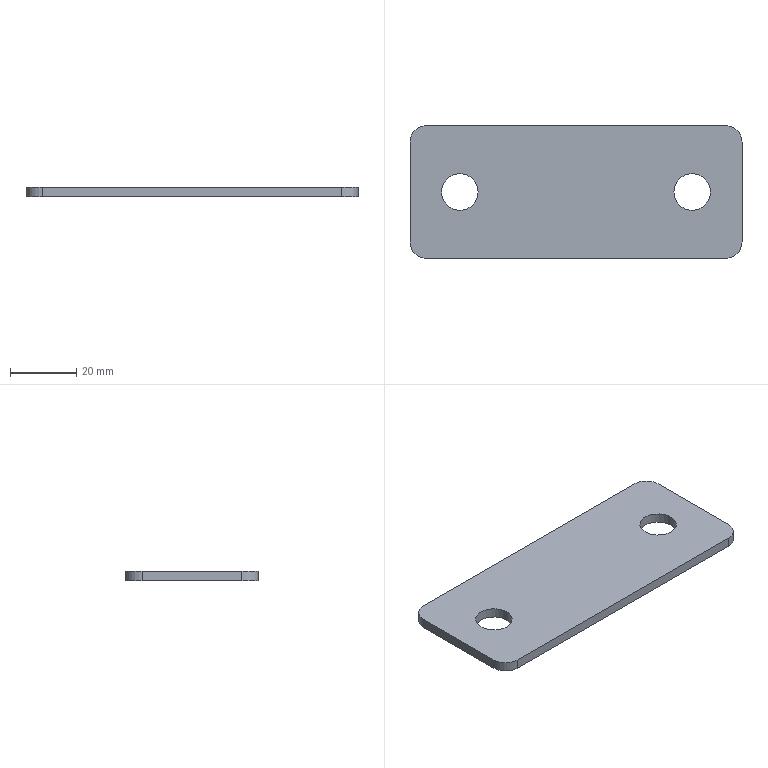Part | STEP file | Part1 | 1 solid | 12 faces | box 100 x 40 x 3 mm | volume 11365 mm3 | cylinder 6 | plane 6 | commonest cylinder face diameters 10 x4 11 x2
STEP:
#1=CARTESIAN_POINT('',(0.,0.,0.));
#2=DIRECTION('',(0.,0.,1.));
#3=DIRECTION('',(1.,0.,0.));
#4=AXIS2_PLACEMENT_3D('',#1,#2,#3);
#5=CARTESIAN_POINT('',(90.5,-20.,3.));
#6=VERTEX_POINT('',#5);
#7=CARTESIAN_POINT('',(85.,-20.,3.));
#8=DIRECTION('',(0.,0.,-1.));
#9=DIRECTION('',(-1.,0.,0.));
#10=AXIS2_PLACEMENT_3D('',#7,#8,#9);
#11=CIRCLE('',#10,5.5);
#12=CARTESIAN_POINT('',(85.,-20.,0.));
#13=DIRECTION('',(0.,0.,1.));
#14=DIRECTION('',(-1.,0.,0.));
#15=AXIS2_PLACEMENT_3D('',#12,#13,#14);
#16=CYLINDRICAL_SURFACE('',#15,5.5);
#17=CARTESIAN_POINT('',(12.566,3.));
#18=DIRECTION('',(-1.,0.));
#19=VECTOR('',#18,1.);
#20=LINE('',#17,#19);
#21=(GEOMETRIC_REPRESENTATION_CONTEXT(2)PARAMETRIC_REPRESENTATION_CONTEXT()REPRESENTATION_CONTEXT('',''));
#22=DEFINITIONAL_REPRESENTATION('',(#20),#21);
#23=PCURVE('',#16,#22);
#24=CARTESIAN_POINT('',(50.,-20.,3.));
#25=DIRECTION('',(0.,0.,1.));
#26=DIRECTION('',(1.,0.,0.));
#27=AXIS2_PLACEMENT_3D('',#24,#25,#26);
#28=PLANE('',#27);
#29=CARTESIAN_POINT('',(29.5,0.));
#30=CARTESIAN_POINT('',(29.5,9.526));
#31=CARTESIAN_POINT('',(37.75,4.763));
#32=CARTESIAN_POINT('',(46.,0.));
#33=CARTESIAN_POINT('',(37.75,-4.763));
#34=CARTESIAN_POINT('',(29.5,-9.526));
#35=CARTESIAN_POINT('',(29.5,0.));
#36=(BOUNDED_CURVE()B_SPLINE_CURVE(2,(#29,#30,#31,#32,#33,#34,#35),.UNSPECIFIED.,.T.,.F.)B_SPLINE_CURVE_WITH_KNOTS((1,2,2,2,2,1),(-2.094,0.,2.094,4.189,6.283,8.378),.UNSPECIFIED.)CURVE()GEOMETRIC_REPRESENTATION_ITEM()RATIONAL_B_SPLINE_CURVE((1.,0.5,1.,0.5,1.,0.5,1.))REPRESENTATION_ITEM(''));
#37=(GEOMETRIC_REPRESENTATION_CONTEXT(2)PARAMETRIC_REPRESENTATION_CONTEXT()REPRESENTATION_CONTEXT('',''));
#38=DEFINITIONAL_REPRESENTATION('',(#36),#37);
#39=PCURVE('',#28,#38);
#40=SURFACE_CURVE('',#11,(#23,#39),.PCURVE_S1.);
#41=EDGE_CURVE('',#6,#6,#40,.T.);
#42=ORIENTED_EDGE('',*,*,#41,.T.);
#43=CARTESIAN_POINT('',(90.5,-20.,0.));
#44=VERTEX_POINT('',#43);
#45=CARTESIAN_POINT('',(90.5,-20.,0.));
#46=CARTESIAN_POINT('',(90.5,-20.,3.));
#47=B_SPLINE_CURVE_WITH_KNOTS('',1,(#45,#46),.UNSPECIFIED.,.F.,.F.,(2,2),(0.,3.),.PIECEWISE_BEZIER_KNOTS.);
#48=CARTESIAN_POINT('',(3.142,0.));
#49=DIRECTION('',(0.,1.));
#50=VECTOR('',#49,1.);
#51=LINE('',#48,#50);
#52=(GEOMETRIC_REPRESENTATION_CONTEXT(2)PARAMETRIC_REPRESENTATION_CONTEXT()REPRESENTATION_CONTEXT('',''));
#53=DEFINITIONAL_REPRESENTATION('',(#51),#52);
#54=PCURVE('',#16,#53);
#55=CARTESIAN_POINT('',(9.425,0.));
#56=DIRECTION('',(0.,1.));
#57=VECTOR('',#56,1.);
#58=LINE('',#55,#57);
#59=(GEOMETRIC_REPRESENTATION_CONTEXT(2)PARAMETRIC_REPRESENTATION_CONTEXT()REPRESENTATION_CONTEXT('',''));
#60=DEFINITIONAL_REPRESENTATION('',(#58),#59);
#61=PCURVE('',#16,#60);
#62=SEAM_CURVE('',#47,(#54,#61),.PCURVE_S1.);
#63=EDGE_CURVE('',#44,#6,#62,.T.);
#64=ORIENTED_EDGE('',*,*,#63,.F.);
#65=CARTESIAN_POINT('',(85.,-20.,0.));
#66=DIRECTION('',(0.,0.,1.));
#67=DIRECTION('',(-1.,0.,0.));
#68=AXIS2_PLACEMENT_3D('',#65,#66,#67);
#69=CIRCLE('',#68,5.5);
#70=CARTESIAN_POINT('',(0.,0.));
#71=DIRECTION('',(1.,0.));
#72=VECTOR('',#71,1.);
#73=LINE('',#70,#72);
#74=(GEOMETRIC_REPRESENTATION_CONTEXT(2)PARAMETRIC_REPRESENTATION_CONTEXT()REPRESENTATION_CONTEXT('',''));
#75=DEFINITIONAL_REPRESENTATION('',(#73),#74);
#76=PCURVE('',#16,#75);
#77=CARTESIAN_POINT('',(50.,-20.,0.));
#78=DIRECTION('',(0.,0.,1.));
#79=DIRECTION('',(1.,0.,0.));
#80=AXIS2_PLACEMENT_3D('',#77,#78,#79);
#81=PLANE('',#80);
#82=CARTESIAN_POINT('',(35.,0.));
#83=DIRECTION('',(-1.,0.));
#84=AXIS2_PLACEMENT_2D('',#82,#83);
#85=CIRCLE('',#84,5.5);
#86=(GEOMETRIC_REPRESENTATION_CONTEXT(2)PARAMETRIC_REPRESENTATION_CONTEXT()REPRESENTATION_CONTEXT('',''));
#87=DEFINITIONAL_REPRESENTATION('',(#85),#86);
#88=PCURVE('',#81,#87);
#89=SURFACE_CURVE('',#69,(#76,#88),.PCURVE_S1.);
#90=EDGE_CURVE('',#44,#44,#89,.T.);
#91=ORIENTED_EDGE('',*,*,#90,.T.);
#92=ORIENTED_EDGE('',*,*,#63,.T.);
#93=EDGE_LOOP('',(#42,#64,#91,#92));
#94=FACE_BOUND('',#93,.F.);
#95=ADVANCED_FACE('',(#94),#16,.F.);
#96=CARTESIAN_POINT('',(20.5,-20.,3.));
#97=VERTEX_POINT('',#96);
#98=CARTESIAN_POINT('',(15.,-20.,3.));
#99=DIRECTION('',(0.,0.,-1.));
#100=DIRECTION('',(-1.,0.,0.));
#101=AXIS2_PLACEMENT_3D('',#98,#99,#100);
#102=CIRCLE('',#101,5.5);
#103=CARTESIAN_POINT('',(15.,-20.,0.));
#104=DIRECTION('',(0.,0.,1.));
#105=DIRECTION('',(-1.,0.,0.));
#106=AXIS2_PLACEMENT_3D('',#103,#104,#105);
#107=CYLINDRICAL_SURFACE('',#106,5.5);
#108=CARTESIAN_POINT('',(12.566,3.));
#109=DIRECTION('',(-1.,0.));
#110=VECTOR('',#109,1.);
#111=LINE('',#108,#110);
#112=(GEOMETRIC_REPRESENTATION_CONTEXT(2)PARAMETRIC_REPRESENTATION_CONTEXT()REPRESENTATION_CONTEXT('',''));
#113=DEFINITIONAL_REPRESENTATION('',(#111),#112);
#114=PCURVE('',#107,#113);
#115=CARTESIAN_POINT('',(-40.5,0.));
#116=CARTESIAN_POINT('',(-40.5,9.526));
#117=CARTESIAN_POINT('',(-32.25,4.763));
#118=CARTESIAN_POINT('',(-24.,0.));
#119=CARTESIAN_POINT('',(-32.25,-4.763));
#120=CARTESIAN_POINT('',(-40.5,-9.526));
#121=CARTESIAN_POINT('',(-40.5,0.));
#122=(BOUNDED_CURVE()B_SPLINE_CURVE(2,(#115,#116,#117,#118,#119,#120,#121),.UNSPECIFIED.,.T.,.F.)B_SPLINE_CURVE_WITH_KNOTS((1,2,2,2,2,1),(-2.094,0.,2.094,4.189,6.283,8.378),.UNSPECIFIED.)CURVE()GEOMETRIC_REPRESENTATION_ITEM()RATIONAL_B_SPLINE_CURVE((1.,0.5,1.,0.5,1.,0.5,1.))REPRESENTATION_ITEM(''));
#123=(GEOMETRIC_REPRESENTATION_CONTEXT(2)PARAMETRIC_REPRESENTATION_CONTEXT()REPRESENTATION_CONTEXT('',''));
#124=DEFINITIONAL_REPRESENTATION('',(#122),#123);
#125=PCURVE('',#28,#124);
#126=SURFACE_CURVE('',#102,(#114,#125),.PCURVE_S1.);
#127=EDGE_CURVE('',#97,#97,#126,.T.);
#128=ORIENTED_EDGE('',*,*,#127,.T.);
#129=CARTESIAN_POINT('',(20.5,-20.,0.));
#130=VERTEX_POINT('',#129);
#131=CARTESIAN_POINT('',(20.5,-20.,0.));
#132=CARTESIAN_POINT('',(20.5,-20.,3.));
#133=B_SPLINE_CURVE_WITH_KNOTS('',1,(#131,#132),.UNSPECIFIED.,.F.,.F.,(2,2),(0.,3.),.PIECEWISE_BEZIER_KNOTS.);
#134=CARTESIAN_POINT('',(3.142,0.));
#135=DIRECTION('',(0.,1.));
#136=VECTOR('',#135,1.);
#137=LINE('',#134,#136);
#138=(GEOMETRIC_REPRESENTATION_CONTEXT(2)PARAMETRIC_REPRESENTATION_CONTEXT()REPRESENTATION_CONTEXT('',''));
#139=DEFINITIONAL_REPRESENTATION('',(#137),#138);
#140=PCURVE('',#107,#139);
#141=CARTESIAN_POINT('',(9.425,0.));
#142=DIRECTION('',(0.,1.));
#143=VECTOR('',#142,1.);
#144=LINE('',#141,#143);
#145=(GEOMETRIC_REPRESENTATION_CONTEXT(2)PARAMETRIC_REPRESENTATION_CONTEXT()REPRESENTATION_CONTEXT('',''));
#146=DEFINITIONAL_REPRESENTATION('',(#144),#145);
#147=PCURVE('',#107,#146);
#148=SEAM_CURVE('',#133,(#140,#147),.PCURVE_S1.);
#149=EDGE_CURVE('',#130,#97,#148,.T.);
#150=ORIENTED_EDGE('',*,*,#149,.F.);
#151=CARTESIAN_POINT('',(15.,-20.,0.));
#152=DIRECTION('',(0.,0.,1.));
#153=DIRECTION('',(-1.,0.,0.));
#154=AXIS2_PLACEMENT_3D('',#151,#152,#153);
#155=CIRCLE('',#154,5.5);
#156=CARTESIAN_POINT('',(0.,0.));
#157=DIRECTION('',(1.,0.));
#158=VECTOR('',#157,1.);
#159=LINE('',#156,#158);
#160=(GEOMETRIC_REPRESENTATION_CONTEXT(2)PARAMETRIC_REPRESENTATION_CONTEXT()REPRESENTATION_CONTEXT('',''));
#161=DEFINITIONAL_REPRESENTATION('',(#159),#160);
#162=PCURVE('',#107,#161);
#163=CARTESIAN_POINT('',(-35.,0.));
#164=DIRECTION('',(-1.,0.));
#165=AXIS2_PLACEMENT_2D('',#163,#164);
#166=CIRCLE('',#165,5.5);
#167=(GEOMETRIC_REPRESENTATION_CONTEXT(2)PARAMETRIC_REPRESENTATION_CONTEXT()REPRESENTATION_CONTEXT('',''));
#168=DEFINITIONAL_REPRESENTATION('',(#166),#167);
#169=PCURVE('',#81,#168);
#170=SURFACE_CURVE('',#155,(#162,#169),.PCURVE_S1.);
#171=EDGE_CURVE('',#130,#130,#170,.T.);
#172=ORIENTED_EDGE('',*,*,#171,.T.);
#173=ORIENTED_EDGE('',*,*,#149,.T.);
#174=EDGE_LOOP('',(#128,#150,#172,#173));
#175=FACE_BOUND('',#174,.F.);
#176=ADVANCED_FACE('',(#175),#107,.F.);
#177=CARTESIAN_POINT('',(5.,0.,0.));
#178=VERTEX_POINT('',#177);
#179=CARTESIAN_POINT('',(0.,-5.,0.));
#180=VERTEX_POINT('',#179);
#181=CARTESIAN_POINT('',(5.,-5.,0.));
#182=DIRECTION('',(0.,0.,1.));
#183=DIRECTION('',(0.,1.,0.));
#184=AXIS2_PLACEMENT_3D('',#181,#182,#183);
#185=CIRCLE('',#184,5.);
#186=CARTESIAN_POINT('',(5.,-5.,0.));
#187=DIRECTION('',(0.,0.,1.));
#188=DIRECTION('',(0.,1.,0.));
#189=AXIS2_PLACEMENT_3D('',#186,#187,#188);
#190=CYLINDRICAL_SURFACE('',#189,5.);
#191=CARTESIAN_POINT('',(0.,0.));
#192=DIRECTION('',(1.,0.));
#193=VECTOR('',#192,1.);
#194=LINE('',#191,#193);
#195=(GEOMETRIC_REPRESENTATION_CONTEXT(2)PARAMETRIC_REPRESENTATION_CONTEXT()REPRESENTATION_CONTEXT('',''));
#196=DEFINITIONAL_REPRESENTATION('',(#194),#195);
#197=PCURVE('',#190,#196);
#198=CARTESIAN_POINT('',(-45.,15.));
#199=DIRECTION('',(0.,1.));
#200=AXIS2_PLACEMENT_2D('',#198,#199);
#201=CIRCLE('',#200,5.);
#202=(GEOMETRIC_REPRESENTATION_CONTEXT(2)PARAMETRIC_REPRESENTATION_CONTEXT()REPRESENTATION_CONTEXT('',''));
#203=DEFINITIONAL_REPRESENTATION('',(#201),#202);
#204=PCURVE('',#81,#203);
#205=SURFACE_CURVE('',#185,(#197,#204),.PCURVE_S1.);
#206=EDGE_CURVE('',#178,#180,#205,.T.);
#207=ORIENTED_EDGE('',*,*,#206,.T.);
#208=CARTESIAN_POINT('',(0.,-5.,3.));
#209=VERTEX_POINT('',#208);
#210=CARTESIAN_POINT('',(0.,-5.,0.));
#211=DIRECTION('',(0.,0.,1.));
#212=VECTOR('',#211,1.);
#213=LINE('',#210,#212);
#214=CARTESIAN_POINT('',(1.571,0.));
#215=DIRECTION('',(0.,1.));
#216=VECTOR('',#215,1.);
#217=LINE('',#214,#216);
#218=(GEOMETRIC_REPRESENTATION_CONTEXT(2)PARAMETRIC_REPRESENTATION_CONTEXT()REPRESENTATION_CONTEXT('',''));
#219=DEFINITIONAL_REPRESENTATION('',(#217),#218);
#220=PCURVE('',#190,#219);
#221=CARTESIAN_POINT('',(0.,-5.,0.));
#222=DIRECTION('',(-1.,0.,0.));
#223=DIRECTION('',(0.,-1.,0.));
#224=AXIS2_PLACEMENT_3D('',#221,#222,#223);
#225=PLANE('',#224);
#226=CARTESIAN_POINT('',(0.,0.));
#227=DIRECTION('',(0.,1.));
#228=VECTOR('',#227,1.);
#229=LINE('',#226,#228);
#230=(GEOMETRIC_REPRESENTATION_CONTEXT(2)PARAMETRIC_REPRESENTATION_CONTEXT()REPRESENTATION_CONTEXT('',''));
#231=DEFINITIONAL_REPRESENTATION('',(#229),#230);
#232=PCURVE('',#225,#231);
#233=SURFACE_CURVE('',#213,(#220,#232),.PCURVE_S1.);
#234=EDGE_CURVE('',#180,#209,#233,.T.);
#235=ORIENTED_EDGE('',*,*,#234,.T.);
#236=CARTESIAN_POINT('',(5.,0.,3.));
#237=VERTEX_POINT('',#236);
#238=CARTESIAN_POINT('',(5.,-5.,3.));
#239=DIRECTION('',(0.,0.,1.));
#240=DIRECTION('',(0.,1.,0.));
#241=AXIS2_PLACEMENT_3D('',#238,#239,#240);
#242=CIRCLE('',#241,5.);
#243=CARTESIAN_POINT('',(0.,3.));
#244=DIRECTION('',(1.,0.));
#245=VECTOR('',#244,1.);
#246=LINE('',#243,#245);
#247=(GEOMETRIC_REPRESENTATION_CONTEXT(2)PARAMETRIC_REPRESENTATION_CONTEXT()REPRESENTATION_CONTEXT('',''));
#248=DEFINITIONAL_REPRESENTATION('',(#246),#247);
#249=PCURVE('',#190,#248);
#250=CARTESIAN_POINT('',(-45.,15.));
#251=DIRECTION('',(0.,1.));
#252=AXIS2_PLACEMENT_2D('',#250,#251);
#253=CIRCLE('',#252,5.);
#254=(GEOMETRIC_REPRESENTATION_CONTEXT(2)PARAMETRIC_REPRESENTATION_CONTEXT()REPRESENTATION_CONTEXT('',''));
#255=DEFINITIONAL_REPRESENTATION('',(#253),#254);
#256=PCURVE('',#28,#255);
#257=SURFACE_CURVE('',#242,(#249,#256),.PCURVE_S1.);
#258=EDGE_CURVE('',#237,#209,#257,.T.);
#259=ORIENTED_EDGE('',*,*,#258,.F.);
#260=CARTESIAN_POINT('',(5.,0.,0.));
#261=DIRECTION('',(0.,0.,1.));
#262=VECTOR('',#261,1.);
#263=LINE('',#260,#262);
#264=CARTESIAN_POINT('',(0.,0.));
#265=DIRECTION('',(0.,1.));
#266=VECTOR('',#265,1.);
#267=LINE('',#264,#266);
#268=(GEOMETRIC_REPRESENTATION_CONTEXT(2)PARAMETRIC_REPRESENTATION_CONTEXT()REPRESENTATION_CONTEXT('',''));
#269=DEFINITIONAL_REPRESENTATION('',(#267),#268);
#270=PCURVE('',#190,#269);
#271=CARTESIAN_POINT('',(95.,0.,0.));
#272=DIRECTION('',(0.,1.,0.));
#273=DIRECTION('',(-1.,0.,0.));
#274=AXIS2_PLACEMENT_3D('',#271,#272,#273);
#275=PLANE('',#274);
#276=CARTESIAN_POINT('',(90.,0.));
#277=DIRECTION('',(0.,1.));
#278=VECTOR('',#277,1.);
#279=LINE('',#276,#278);
#280=(GEOMETRIC_REPRESENTATION_CONTEXT(2)PARAMETRIC_REPRESENTATION_CONTEXT()REPRESENTATION_CONTEXT('',''));
#281=DEFINITIONAL_REPRESENTATION('',(#279),#280);
#282=PCURVE('',#275,#281);
#283=SURFACE_CURVE('',#263,(#270,#282),.PCURVE_S1.);
#284=EDGE_CURVE('',#178,#237,#283,.T.);
#285=ORIENTED_EDGE('',*,*,#284,.F.);
#286=EDGE_LOOP('',(#207,#235,#259,#285));
#287=FACE_BOUND('',#286,.T.);
#288=ADVANCED_FACE('',(#287),#190,.T.);
#289=CARTESIAN_POINT('',(95.,0.,0.));
#290=VERTEX_POINT('',#289);
#291=CARTESIAN_POINT('',(95.,0.,0.));
#292=DIRECTION('',(-1.,0.,0.));
#293=VECTOR('',#292,1.);
#294=LINE('',#291,#293);
#295=CARTESIAN_POINT('',(0.,0.));
#296=DIRECTION('',(1.,0.));
#297=VECTOR('',#296,1.);
#298=LINE('',#295,#297);
#299=(GEOMETRIC_REPRESENTATION_CONTEXT(2)PARAMETRIC_REPRESENTATION_CONTEXT()REPRESENTATION_CONTEXT('',''));
#300=DEFINITIONAL_REPRESENTATION('',(#298),#299);
#301=PCURVE('',#275,#300);
#302=CARTESIAN_POINT('',(45.,20.));
#303=DIRECTION('',(-1.,0.));
#304=VECTOR('',#303,1.);
#305=LINE('',#302,#304);
#306=(GEOMETRIC_REPRESENTATION_CONTEXT(2)PARAMETRIC_REPRESENTATION_CONTEXT()REPRESENTATION_CONTEXT('',''));
#307=DEFINITIONAL_REPRESENTATION('',(#305),#306);
#308=PCURVE('',#81,#307);
#309=SURFACE_CURVE('',#294,(#301,#308),.PCURVE_S1.);
#310=EDGE_CURVE('',#290,#178,#309,.T.);
#311=ORIENTED_EDGE('',*,*,#310,.T.);
#312=ORIENTED_EDGE('',*,*,#284,.T.);
#313=CARTESIAN_POINT('',(95.,0.,3.));
#314=VERTEX_POINT('',#313);
#315=CARTESIAN_POINT('',(95.,0.,3.));
#316=DIRECTION('',(-1.,0.,0.));
#317=VECTOR('',#316,1.);
#318=LINE('',#315,#317);
#319=CARTESIAN_POINT('',(0.,3.));
#320=DIRECTION('',(1.,0.));
#321=VECTOR('',#320,1.);
#322=LINE('',#319,#321);
#323=(GEOMETRIC_REPRESENTATION_CONTEXT(2)PARAMETRIC_REPRESENTATION_CONTEXT()REPRESENTATION_CONTEXT('',''));
#324=DEFINITIONAL_REPRESENTATION('',(#322),#323);
#325=PCURVE('',#275,#324);
#326=CARTESIAN_POINT('',(45.,20.));
#327=DIRECTION('',(-1.,0.));
#328=VECTOR('',#327,1.);
#329=LINE('',#326,#328);
#330=(GEOMETRIC_REPRESENTATION_CONTEXT(2)PARAMETRIC_REPRESENTATION_CONTEXT()REPRESENTATION_CONTEXT('',''));
#331=DEFINITIONAL_REPRESENTATION('',(#329),#330);
#332=PCURVE('',#28,#331);
#333=SURFACE_CURVE('',#318,(#325,#332),.PCURVE_S1.);
#334=EDGE_CURVE('',#314,#237,#333,.T.);
#335=ORIENTED_EDGE('',*,*,#334,.F.);
#336=CARTESIAN_POINT('',(95.,0.,0.));
#337=DIRECTION('',(0.,0.,1.));
#338=VECTOR('',#337,1.);
#339=LINE('',#336,#338);
#340=CARTESIAN_POINT('',(0.,0.));
#341=DIRECTION('',(0.,1.));
#342=VECTOR('',#341,1.);
#343=LINE('',#340,#342);
#344=(GEOMETRIC_REPRESENTATION_CONTEXT(2)PARAMETRIC_REPRESENTATION_CONTEXT()REPRESENTATION_CONTEXT('',''));
#345=DEFINITIONAL_REPRESENTATION('',(#343),#344);
#346=PCURVE('',#275,#345);
#347=CARTESIAN_POINT('',(95.,-5.,0.));
#348=DIRECTION('',(0.,0.,1.));
#349=DIRECTION('',(1.,0.,0.));
#350=AXIS2_PLACEMENT_3D('',#347,#348,#349);
#351=CYLINDRICAL_SURFACE('',#350,5.);
#352=CARTESIAN_POINT('',(1.571,0.));
#353=DIRECTION('',(0.,1.));
#354=VECTOR('',#353,1.);
#355=LINE('',#352,#354);
#356=(GEOMETRIC_REPRESENTATION_CONTEXT(2)PARAMETRIC_REPRESENTATION_CONTEXT()REPRESENTATION_CONTEXT('',''));
#357=DEFINITIONAL_REPRESENTATION('',(#355),#356);
#358=PCURVE('',#351,#357);
#359=SURFACE_CURVE('',#339,(#346,#358),.PCURVE_S1.);
#360=EDGE_CURVE('',#290,#314,#359,.T.);
#361=ORIENTED_EDGE('',*,*,#360,.F.);
#362=EDGE_LOOP('',(#311,#312,#335,#361));
#363=FACE_BOUND('',#362,.T.);
#364=ADVANCED_FACE('',(#363),#275,.T.);
#365=CARTESIAN_POINT('',(100.,-5.,0.));
#366=VERTEX_POINT('',#365);
#367=CARTESIAN_POINT('',(95.,-5.,0.));
#368=DIRECTION('',(0.,0.,1.));
#369=DIRECTION('',(1.,0.,0.));
#370=AXIS2_PLACEMENT_3D('',#367,#368,#369);
#371=CIRCLE('',#370,5.);
#372=CARTESIAN_POINT('',(0.,0.));
#373=DIRECTION('',(1.,0.));
#374=VECTOR('',#373,1.);
#375=LINE('',#372,#374);
#376=(GEOMETRIC_REPRESENTATION_CONTEXT(2)PARAMETRIC_REPRESENTATION_CONTEXT()REPRESENTATION_CONTEXT('',''));
#377=DEFINITIONAL_REPRESENTATION('',(#375),#376);
#378=PCURVE('',#351,#377);
#379=CARTESIAN_POINT('',(45.,15.));
#380=DIRECTION('',(1.,0.));
#381=AXIS2_PLACEMENT_2D('',#379,#380);
#382=CIRCLE('',#381,5.);
#383=(GEOMETRIC_REPRESENTATION_CONTEXT(2)PARAMETRIC_REPRESENTATION_CONTEXT()REPRESENTATION_CONTEXT('',''));
#384=DEFINITIONAL_REPRESENTATION('',(#382),#383);
#385=PCURVE('',#81,#384);
#386=SURFACE_CURVE('',#371,(#378,#385),.PCURVE_S1.);
#387=EDGE_CURVE('',#366,#290,#386,.T.);
#388=ORIENTED_EDGE('',*,*,#387,.T.);
#389=ORIENTED_EDGE('',*,*,#360,.T.);
#390=CARTESIAN_POINT('',(100.,-5.,3.));
#391=VERTEX_POINT('',#390);
#392=CARTESIAN_POINT('',(95.,-5.,3.));
#393=DIRECTION('',(0.,0.,1.));
#394=DIRECTION('',(1.,0.,0.));
#395=AXIS2_PLACEMENT_3D('',#392,#393,#394);
#396=CIRCLE('',#395,5.);
#397=CARTESIAN_POINT('',(0.,3.));
#398=DIRECTION('',(1.,0.));
#399=VECTOR('',#398,1.);
#400=LINE('',#397,#399);
#401=(GEOMETRIC_REPRESENTATION_CONTEXT(2)PARAMETRIC_REPRESENTATION_CONTEXT()REPRESENTATION_CONTEXT('',''));
#402=DEFINITIONAL_REPRESENTATION('',(#400),#401);
#403=PCURVE('',#351,#402);
#404=CARTESIAN_POINT('',(45.,15.));
#405=DIRECTION('',(1.,0.));
#406=AXIS2_PLACEMENT_2D('',#404,#405);
#407=CIRCLE('',#406,5.);
#408=(GEOMETRIC_REPRESENTATION_CONTEXT(2)PARAMETRIC_REPRESENTATION_CONTEXT()REPRESENTATION_CONTEXT('',''));
#409=DEFINITIONAL_REPRESENTATION('',(#407),#408);
#410=PCURVE('',#28,#409);
#411=SURFACE_CURVE('',#396,(#403,#410),.PCURVE_S1.);
#412=EDGE_CURVE('',#391,#314,#411,.T.);
#413=ORIENTED_EDGE('',*,*,#412,.F.);
#414=CARTESIAN_POINT('',(100.,-5.,0.));
#415=DIRECTION('',(0.,0.,1.));
#416=VECTOR('',#415,1.);
#417=LINE('',#414,#416);
#418=CARTESIAN_POINT('',(0.,0.));
#419=DIRECTION('',(0.,1.));
#420=VECTOR('',#419,1.);
#421=LINE('',#418,#420);
#422=(GEOMETRIC_REPRESENTATION_CONTEXT(2)PARAMETRIC_REPRESENTATION_CONTEXT()REPRESENTATION_CONTEXT('',''));
#423=DEFINITIONAL_REPRESENTATION('',(#421),#422);
#424=PCURVE('',#351,#423);
#425=CARTESIAN_POINT('',(100.,-35.,0.));
#426=DIRECTION('',(1.,0.,0.));
#427=DIRECTION('',(0.,1.,0.));
#428=AXIS2_PLACEMENT_3D('',#425,#426,#427);
#429=PLANE('',#428);
#430=CARTESIAN_POINT('',(30.,0.));
#431=DIRECTION('',(0.,1.));
#432=VECTOR('',#431,1.);
#433=LINE('',#430,#432);
#434=(GEOMETRIC_REPRESENTATION_CONTEXT(2)PARAMETRIC_REPRESENTATION_CONTEXT()REPRESENTATION_CONTEXT('',''));
#435=DEFINITIONAL_REPRESENTATION('',(#433),#434);
#436=PCURVE('',#429,#435);
#437=SURFACE_CURVE('',#417,(#424,#436),.PCURVE_S1.);
#438=EDGE_CURVE('',#366,#391,#437,.T.);
#439=ORIENTED_EDGE('',*,*,#438,.F.);
#440=EDGE_LOOP('',(#388,#389,#413,#439));
#441=FACE_BOUND('',#440,.T.);
#442=ADVANCED_FACE('',(#441),#351,.T.);
#443=CARTESIAN_POINT('',(100.,-35.,0.));
#444=VERTEX_POINT('',#443);
#445=CARTESIAN_POINT('',(100.,-35.,0.));
#446=DIRECTION('',(0.,1.,0.));
#447=VECTOR('',#446,1.);
#448=LINE('',#445,#447);
#449=CARTESIAN_POINT('',(0.,0.));
#450=DIRECTION('',(1.,0.));
#451=VECTOR('',#450,1.);
#452=LINE('',#449,#451);
#453=(GEOMETRIC_REPRESENTATION_CONTEXT(2)PARAMETRIC_REPRESENTATION_CONTEXT()REPRESENTATION_CONTEXT('',''));
#454=DEFINITIONAL_REPRESENTATION('',(#452),#453);
#455=PCURVE('',#429,#454);
#456=CARTESIAN_POINT('',(50.,-15.));
#457=DIRECTION('',(0.,1.));
#458=VECTOR('',#457,1.);
#459=LINE('',#456,#458);
#460=(GEOMETRIC_REPRESENTATION_CONTEXT(2)PARAMETRIC_REPRESENTATION_CONTEXT()REPRESENTATION_CONTEXT('',''));
#461=DEFINITIONAL_REPRESENTATION('',(#459),#460);
#462=PCURVE('',#81,#461);
#463=SURFACE_CURVE('',#448,(#455,#462),.PCURVE_S1.);
#464=EDGE_CURVE('',#444,#366,#463,.T.);
#465=ORIENTED_EDGE('',*,*,#464,.T.);
#466=ORIENTED_EDGE('',*,*,#438,.T.);
#467=CARTESIAN_POINT('',(100.,-35.,3.));
#468=VERTEX_POINT('',#467);
#469=CARTESIAN_POINT('',(100.,-35.,3.));
#470=DIRECTION('',(0.,1.,0.));
#471=VECTOR('',#470,1.);
#472=LINE('',#469,#471);
#473=CARTESIAN_POINT('',(0.,3.));
#474=DIRECTION('',(1.,0.));
#475=VECTOR('',#474,1.);
#476=LINE('',#473,#475);
#477=(GEOMETRIC_REPRESENTATION_CONTEXT(2)PARAMETRIC_REPRESENTATION_CONTEXT()REPRESENTATION_CONTEXT('',''));
#478=DEFINITIONAL_REPRESENTATION('',(#476),#477);
#479=PCURVE('',#429,#478);
#480=CARTESIAN_POINT('',(50.,-15.));
#481=DIRECTION('',(0.,1.));
#482=VECTOR('',#481,1.);
#483=LINE('',#480,#482);
#484=(GEOMETRIC_REPRESENTATION_CONTEXT(2)PARAMETRIC_REPRESENTATION_CONTEXT()REPRESENTATION_CONTEXT('',''));
#485=DEFINITIONAL_REPRESENTATION('',(#483),#484);
#486=PCURVE('',#28,#485);
#487=SURFACE_CURVE('',#472,(#479,#486),.PCURVE_S1.);
#488=EDGE_CURVE('',#468,#391,#487,.T.);
#489=ORIENTED_EDGE('',*,*,#488,.F.);
#490=CARTESIAN_POINT('',(100.,-35.,0.));
#491=DIRECTION('',(0.,0.,1.));
#492=VECTOR('',#491,1.);
#493=LINE('',#490,#492);
#494=CARTESIAN_POINT('',(0.,0.));
#495=DIRECTION('',(0.,1.));
#496=VECTOR('',#495,1.);
#497=LINE('',#494,#496);
#498=(GEOMETRIC_REPRESENTATION_CONTEXT(2)PARAMETRIC_REPRESENTATION_CONTEXT()REPRESENTATION_CONTEXT('',''));
#499=DEFINITIONAL_REPRESENTATION('',(#497),#498);
#500=PCURVE('',#429,#499);
#501=CARTESIAN_POINT('',(95.,-35.,0.));
#502=DIRECTION('',(0.,0.,1.));
#503=DIRECTION('',(0.,-1.,0.));
#504=AXIS2_PLACEMENT_3D('',#501,#502,#503);
#505=CYLINDRICAL_SURFACE('',#504,5.);
#506=CARTESIAN_POINT('',(1.571,0.));
#507=DIRECTION('',(0.,1.));
#508=VECTOR('',#507,1.);
#509=LINE('',#506,#508);
#510=(GEOMETRIC_REPRESENTATION_CONTEXT(2)PARAMETRIC_REPRESENTATION_CONTEXT()REPRESENTATION_CONTEXT('',''));
#511=DEFINITIONAL_REPRESENTATION('',(#509),#510);
#512=PCURVE('',#505,#511);
#513=SURFACE_CURVE('',#493,(#500,#512),.PCURVE_S1.);
#514=EDGE_CURVE('',#444,#468,#513,.T.);
#515=ORIENTED_EDGE('',*,*,#514,.F.);
#516=EDGE_LOOP('',(#465,#466,#489,#515));
#517=FACE_BOUND('',#516,.T.);
#518=ADVANCED_FACE('',(#517),#429,.T.);
#519=CARTESIAN_POINT('',(95.,-40.,0.));
#520=VERTEX_POINT('',#519);
#521=CARTESIAN_POINT('',(95.,-35.,0.));
#522=DIRECTION('',(0.,0.,1.));
#523=DIRECTION('',(0.,-1.,0.));
#524=AXIS2_PLACEMENT_3D('',#521,#522,#523);
#525=CIRCLE('',#524,5.);
#526=CARTESIAN_POINT('',(0.,0.));
#527=DIRECTION('',(1.,0.));
#528=VECTOR('',#527,1.);
#529=LINE('',#526,#528);
#530=(GEOMETRIC_REPRESENTATION_CONTEXT(2)PARAMETRIC_REPRESENTATION_CONTEXT()REPRESENTATION_CONTEXT('',''));
#531=DEFINITIONAL_REPRESENTATION('',(#529),#530);
#532=PCURVE('',#505,#531);
#533=CARTESIAN_POINT('',(45.,-15.));
#534=DIRECTION('',(0.,-1.));
#535=AXIS2_PLACEMENT_2D('',#533,#534);
#536=CIRCLE('',#535,5.);
#537=(GEOMETRIC_REPRESENTATION_CONTEXT(2)PARAMETRIC_REPRESENTATION_CONTEXT()REPRESENTATION_CONTEXT('',''));
#538=DEFINITIONAL_REPRESENTATION('',(#536),#537);
#539=PCURVE('',#81,#538);
#540=SURFACE_CURVE('',#525,(#532,#539),.PCURVE_S1.);
#541=EDGE_CURVE('',#520,#444,#540,.T.);
#542=ORIENTED_EDGE('',*,*,#541,.T.);
#543=ORIENTED_EDGE('',*,*,#514,.T.);
#544=CARTESIAN_POINT('',(95.,-40.,3.));
#545=VERTEX_POINT('',#544);
#546=CARTESIAN_POINT('',(95.,-35.,3.));
#547=DIRECTION('',(0.,0.,1.));
#548=DIRECTION('',(0.,-1.,0.));
#549=AXIS2_PLACEMENT_3D('',#546,#547,#548);
#550=CIRCLE('',#549,5.);
#551=CARTESIAN_POINT('',(0.,3.));
#552=DIRECTION('',(1.,0.));
#553=VECTOR('',#552,1.);
#554=LINE('',#551,#553);
#555=(GEOMETRIC_REPRESENTATION_CONTEXT(2)PARAMETRIC_REPRESENTATION_CONTEXT()REPRESENTATION_CONTEXT('',''));
#556=DEFINITIONAL_REPRESENTATION('',(#554),#555);
#557=PCURVE('',#505,#556);
#558=CARTESIAN_POINT('',(45.,-15.));
#559=DIRECTION('',(0.,-1.));
#560=AXIS2_PLACEMENT_2D('',#558,#559);
#561=CIRCLE('',#560,5.);
#562=(GEOMETRIC_REPRESENTATION_CONTEXT(2)PARAMETRIC_REPRESENTATION_CONTEXT()REPRESENTATION_CONTEXT('',''));
#563=DEFINITIONAL_REPRESENTATION('',(#561),#562);
#564=PCURVE('',#28,#563);
#565=SURFACE_CURVE('',#550,(#557,#564),.PCURVE_S1.);
#566=EDGE_CURVE('',#545,#468,#565,.T.);
#567=ORIENTED_EDGE('',*,*,#566,.F.);
#568=CARTESIAN_POINT('',(95.,-40.,0.));
#569=DIRECTION('',(0.,0.,1.));
#570=VECTOR('',#569,1.);
#571=LINE('',#568,#570);
#572=CARTESIAN_POINT('',(0.,0.));
#573=DIRECTION('',(0.,1.));
#574=VECTOR('',#573,1.);
#575=LINE('',#572,#574);
#576=(GEOMETRIC_REPRESENTATION_CONTEXT(2)PARAMETRIC_REPRESENTATION_CONTEXT()REPRESENTATION_CONTEXT('',''));
#577=DEFINITIONAL_REPRESENTATION('',(#575),#576);
#578=PCURVE('',#505,#577);
#579=CARTESIAN_POINT('',(5.,-40.,0.));
#580=DIRECTION('',(0.,-1.,0.));
#581=DIRECTION('',(1.,0.,0.));
#582=AXIS2_PLACEMENT_3D('',#579,#580,#581);
#583=PLANE('',#582);
#584=CARTESIAN_POINT('',(90.,0.));
#585=DIRECTION('',(0.,1.));
#586=VECTOR('',#585,1.);
#587=LINE('',#584,#586);
#588=(GEOMETRIC_REPRESENTATION_CONTEXT(2)PARAMETRIC_REPRESENTATION_CONTEXT()REPRESENTATION_CONTEXT('',''));
#589=DEFINITIONAL_REPRESENTATION('',(#587),#588);
#590=PCURVE('',#583,#589);
#591=SURFACE_CURVE('',#571,(#578,#590),.PCURVE_S1.);
#592=EDGE_CURVE('',#520,#545,#591,.T.);
#593=ORIENTED_EDGE('',*,*,#592,.F.);
#594=EDGE_LOOP('',(#542,#543,#567,#593));
#595=FACE_BOUND('',#594,.T.);
#596=ADVANCED_FACE('',(#595),#505,.T.);
#597=CARTESIAN_POINT('',(5.,-40.,0.));
#598=VERTEX_POINT('',#597);
#599=CARTESIAN_POINT('',(5.,-40.,0.));
#600=DIRECTION('',(1.,0.,0.));
#601=VECTOR('',#600,1.);
#602=LINE('',#599,#601);
#603=CARTESIAN_POINT('',(0.,0.));
#604=DIRECTION('',(1.,0.));
#605=VECTOR('',#604,1.);
#606=LINE('',#603,#605);
#607=(GEOMETRIC_REPRESENTATION_CONTEXT(2)PARAMETRIC_REPRESENTATION_CONTEXT()REPRESENTATION_CONTEXT('',''));
#608=DEFINITIONAL_REPRESENTATION('',(#606),#607);
#609=PCURVE('',#583,#608);
#610=CARTESIAN_POINT('',(-45.,-20.));
#611=DIRECTION('',(1.,0.));
#612=VECTOR('',#611,1.);
#613=LINE('',#610,#612);
#614=(GEOMETRIC_REPRESENTATION_CONTEXT(2)PARAMETRIC_REPRESENTATION_CONTEXT()REPRESENTATION_CONTEXT('',''));
#615=DEFINITIONAL_REPRESENTATION('',(#613),#614);
#616=PCURVE('',#81,#615);
#617=SURFACE_CURVE('',#602,(#609,#616),.PCURVE_S1.);
#618=EDGE_CURVE('',#598,#520,#617,.T.);
#619=ORIENTED_EDGE('',*,*,#618,.T.);
#620=ORIENTED_EDGE('',*,*,#592,.T.);
#621=CARTESIAN_POINT('',(5.,-40.,3.));
#622=VERTEX_POINT('',#621);
#623=CARTESIAN_POINT('',(5.,-40.,3.));
#624=DIRECTION('',(1.,0.,0.));
#625=VECTOR('',#624,1.);
#626=LINE('',#623,#625);
#627=CARTESIAN_POINT('',(0.,3.));
#628=DIRECTION('',(1.,0.));
#629=VECTOR('',#628,1.);
#630=LINE('',#627,#629);
#631=(GEOMETRIC_REPRESENTATION_CONTEXT(2)PARAMETRIC_REPRESENTATION_CONTEXT()REPRESENTATION_CONTEXT('',''));
#632=DEFINITIONAL_REPRESENTATION('',(#630),#631);
#633=PCURVE('',#583,#632);
#634=CARTESIAN_POINT('',(-45.,-20.));
#635=DIRECTION('',(1.,0.));
#636=VECTOR('',#635,1.);
#637=LINE('',#634,#636);
#638=(GEOMETRIC_REPRESENTATION_CONTEXT(2)PARAMETRIC_REPRESENTATION_CONTEXT()REPRESENTATION_CONTEXT('',''));
#639=DEFINITIONAL_REPRESENTATION('',(#637),#638);
#640=PCURVE('',#28,#639);
#641=SURFACE_CURVE('',#626,(#633,#640),.PCURVE_S1.);
#642=EDGE_CURVE('',#622,#545,#641,.T.);
#643=ORIENTED_EDGE('',*,*,#642,.F.);
#644=CARTESIAN_POINT('',(5.,-40.,0.));
#645=DIRECTION('',(0.,0.,1.));
#646=VECTOR('',#645,1.);
#647=LINE('',#644,#646);
#648=CARTESIAN_POINT('',(0.,0.));
#649=DIRECTION('',(0.,1.));
#650=VECTOR('',#649,1.);
#651=LINE('',#648,#650);
#652=(GEOMETRIC_REPRESENTATION_CONTEXT(2)PARAMETRIC_REPRESENTATION_CONTEXT()REPRESENTATION_CONTEXT('',''));
#653=DEFINITIONAL_REPRESENTATION('',(#651),#652);
#654=PCURVE('',#583,#653);
#655=CARTESIAN_POINT('',(5.,-35.,0.));
#656=DIRECTION('',(0.,0.,1.));
#657=DIRECTION('',(-1.,0.,0.));
#658=AXIS2_PLACEMENT_3D('',#655,#656,#657);
#659=CYLINDRICAL_SURFACE('',#658,5.);
#660=CARTESIAN_POINT('',(1.571,0.));
#661=DIRECTION('',(0.,1.));
#662=VECTOR('',#661,1.);
#663=LINE('',#660,#662);
#664=(GEOMETRIC_REPRESENTATION_CONTEXT(2)PARAMETRIC_REPRESENTATION_CONTEXT()REPRESENTATION_CONTEXT('',''));
#665=DEFINITIONAL_REPRESENTATION('',(#663),#664);
#666=PCURVE('',#659,#665);
#667=SURFACE_CURVE('',#647,(#654,#666),.PCURVE_S1.);
#668=EDGE_CURVE('',#598,#622,#667,.T.);
#669=ORIENTED_EDGE('',*,*,#668,.F.);
#670=EDGE_LOOP('',(#619,#620,#643,#669));
#671=FACE_BOUND('',#670,.T.);
#672=ADVANCED_FACE('',(#671),#583,.T.);
#673=CARTESIAN_POINT('',(0.,-35.,0.));
#674=VERTEX_POINT('',#673);
#675=CARTESIAN_POINT('',(5.,-35.,0.));
#676=DIRECTION('',(0.,0.,1.));
#677=DIRECTION('',(-1.,0.,0.));
#678=AXIS2_PLACEMENT_3D('',#675,#676,#677);
#679=CIRCLE('',#678,5.);
#680=CARTESIAN_POINT('',(0.,0.));
#681=DIRECTION('',(1.,0.));
#682=VECTOR('',#681,1.);
#683=LINE('',#680,#682);
#684=(GEOMETRIC_REPRESENTATION_CONTEXT(2)PARAMETRIC_REPRESENTATION_CONTEXT()REPRESENTATION_CONTEXT('',''));
#685=DEFINITIONAL_REPRESENTATION('',(#683),#684);
#686=PCURVE('',#659,#685);
#687=CARTESIAN_POINT('',(-45.,-15.));
#688=DIRECTION('',(-1.,0.));
#689=AXIS2_PLACEMENT_2D('',#687,#688);
#690=CIRCLE('',#689,5.);
#691=(GEOMETRIC_REPRESENTATION_CONTEXT(2)PARAMETRIC_REPRESENTATION_CONTEXT()REPRESENTATION_CONTEXT('',''));
#692=DEFINITIONAL_REPRESENTATION('',(#690),#691);
#693=PCURVE('',#81,#692);
#694=SURFACE_CURVE('',#679,(#686,#693),.PCURVE_S1.);
#695=EDGE_CURVE('',#674,#598,#694,.T.);
#696=ORIENTED_EDGE('',*,*,#695,.T.);
#697=ORIENTED_EDGE('',*,*,#668,.T.);
#698=CARTESIAN_POINT('',(0.,-35.,3.));
#699=VERTEX_POINT('',#698);
#700=CARTESIAN_POINT('',(5.,-35.,3.));
#701=DIRECTION('',(0.,0.,1.));
#702=DIRECTION('',(-1.,0.,0.));
#703=AXIS2_PLACEMENT_3D('',#700,#701,#702);
#704=CIRCLE('',#703,5.);
#705=CARTESIAN_POINT('',(0.,3.));
#706=DIRECTION('',(1.,0.));
#707=VECTOR('',#706,1.);
#708=LINE('',#705,#707);
#709=(GEOMETRIC_REPRESENTATION_CONTEXT(2)PARAMETRIC_REPRESENTATION_CONTEXT()REPRESENTATION_CONTEXT('',''));
#710=DEFINITIONAL_REPRESENTATION('',(#708),#709);
#711=PCURVE('',#659,#710);
#712=CARTESIAN_POINT('',(-45.,-15.));
#713=DIRECTION('',(-1.,0.));
#714=AXIS2_PLACEMENT_2D('',#712,#713);
#715=CIRCLE('',#714,5.);
#716=(GEOMETRIC_REPRESENTATION_CONTEXT(2)PARAMETRIC_REPRESENTATION_CONTEXT()REPRESENTATION_CONTEXT('',''));
#717=DEFINITIONAL_REPRESENTATION('',(#715),#716);
#718=PCURVE('',#28,#717);
#719=SURFACE_CURVE('',#704,(#711,#718),.PCURVE_S1.);
#720=EDGE_CURVE('',#699,#622,#719,.T.);
#721=ORIENTED_EDGE('',*,*,#720,.F.);
#722=CARTESIAN_POINT('',(0.,-35.,0.));
#723=DIRECTION('',(0.,0.,1.));
#724=VECTOR('',#723,1.);
#725=LINE('',#722,#724);
#726=CARTESIAN_POINT('',(0.,0.));
#727=DIRECTION('',(0.,1.));
#728=VECTOR('',#727,1.);
#729=LINE('',#726,#728);
#730=(GEOMETRIC_REPRESENTATION_CONTEXT(2)PARAMETRIC_REPRESENTATION_CONTEXT()REPRESENTATION_CONTEXT('',''));
#731=DEFINITIONAL_REPRESENTATION('',(#729),#730);
#732=PCURVE('',#659,#731);
#733=CARTESIAN_POINT('',(30.,0.));
#734=DIRECTION('',(0.,1.));
#735=VECTOR('',#734,1.);
#736=LINE('',#733,#735);
#737=(GEOMETRIC_REPRESENTATION_CONTEXT(2)PARAMETRIC_REPRESENTATION_CONTEXT()REPRESENTATION_CONTEXT('',''));
#738=DEFINITIONAL_REPRESENTATION('',(#736),#737);
#739=PCURVE('',#225,#738);
#740=SURFACE_CURVE('',#725,(#732,#739),.PCURVE_S1.);
#741=EDGE_CURVE('',#674,#699,#740,.T.);
#742=ORIENTED_EDGE('',*,*,#741,.F.);
#743=EDGE_LOOP('',(#696,#697,#721,#742));
#744=FACE_BOUND('',#743,.T.);
#745=ADVANCED_FACE('',(#744),#659,.T.);
#746=CARTESIAN_POINT('',(0.,-5.,0.));
#747=DIRECTION('',(0.,-1.,0.));
#748=VECTOR('',#747,1.);
#749=LINE('',#746,#748);
#750=CARTESIAN_POINT('',(0.,0.));
#751=DIRECTION('',(1.,0.));
#752=VECTOR('',#751,1.);
#753=LINE('',#750,#752);
#754=(GEOMETRIC_REPRESENTATION_CONTEXT(2)PARAMETRIC_REPRESENTATION_CONTEXT()REPRESENTATION_CONTEXT('',''));
#755=DEFINITIONAL_REPRESENTATION('',(#753),#754);
#756=PCURVE('',#225,#755);
#757=CARTESIAN_POINT('',(-50.,15.));
#758=DIRECTION('',(0.,-1.));
#759=VECTOR('',#758,1.);
#760=LINE('',#757,#759);
#761=(GEOMETRIC_REPRESENTATION_CONTEXT(2)PARAMETRIC_REPRESENTATION_CONTEXT()REPRESENTATION_CONTEXT('',''));
#762=DEFINITIONAL_REPRESENTATION('',(#760),#761);
#763=PCURVE('',#81,#762);
#764=SURFACE_CURVE('',#749,(#756,#763),.PCURVE_S1.);
#765=EDGE_CURVE('',#180,#674,#764,.T.);
#766=ORIENTED_EDGE('',*,*,#765,.T.);
#767=ORIENTED_EDGE('',*,*,#741,.T.);
#768=CARTESIAN_POINT('',(0.,-5.,3.));
#769=DIRECTION('',(0.,-1.,0.));
#770=VECTOR('',#769,1.);
#771=LINE('',#768,#770);
#772=CARTESIAN_POINT('',(0.,3.));
#773=DIRECTION('',(1.,0.));
#774=VECTOR('',#773,1.);
#775=LINE('',#772,#774);
#776=(GEOMETRIC_REPRESENTATION_CONTEXT(2)PARAMETRIC_REPRESENTATION_CONTEXT()REPRESENTATION_CONTEXT('',''));
#777=DEFINITIONAL_REPRESENTATION('',(#775),#776);
#778=PCURVE('',#225,#777);
#779=CARTESIAN_POINT('',(-50.,15.));
#780=DIRECTION('',(0.,-1.));
#781=VECTOR('',#780,1.);
#782=LINE('',#779,#781);
#783=(GEOMETRIC_REPRESENTATION_CONTEXT(2)PARAMETRIC_REPRESENTATION_CONTEXT()REPRESENTATION_CONTEXT('',''));
#784=DEFINITIONAL_REPRESENTATION('',(#782),#783);
#785=PCURVE('',#28,#784);
#786=SURFACE_CURVE('',#771,(#778,#785),.PCURVE_S1.);
#787=EDGE_CURVE('',#209,#699,#786,.T.);
#788=ORIENTED_EDGE('',*,*,#787,.F.);
#789=ORIENTED_EDGE('',*,*,#234,.F.);
#790=EDGE_LOOP('',(#766,#767,#788,#789));
#791=FACE_BOUND('',#790,.T.);
#792=ADVANCED_FACE('',(#791),#225,.T.);
#793=ORIENTED_EDGE('',*,*,#787,.T.);
#794=ORIENTED_EDGE('',*,*,#720,.T.);
#795=ORIENTED_EDGE('',*,*,#642,.T.);
#796=ORIENTED_EDGE('',*,*,#566,.T.);
#797=ORIENTED_EDGE('',*,*,#488,.T.);
#798=ORIENTED_EDGE('',*,*,#412,.T.);
#799=ORIENTED_EDGE('',*,*,#334,.T.);
#800=ORIENTED_EDGE('',*,*,#258,.T.);
#801=EDGE_LOOP('',(#793,#794,#795,#796,#797,#798,#799,#800));
#802=FACE_BOUND('',#801,.T.);
#803=ORIENTED_EDGE('',*,*,#41,.T.);
#804=EDGE_LOOP('',(#803));
#805=FACE_BOUND('',#804,.T.);
#806=ORIENTED_EDGE('',*,*,#127,.T.);
#807=EDGE_LOOP('',(#806));
#808=FACE_BOUND('',#807,.T.);
#809=ADVANCED_FACE('',(#802,#805,#808),#28,.T.);
#810=ORIENTED_EDGE('',*,*,#765,.F.);
#811=ORIENTED_EDGE('',*,*,#206,.F.);
#812=ORIENTED_EDGE('',*,*,#310,.F.);
#813=ORIENTED_EDGE('',*,*,#387,.F.);
#814=ORIENTED_EDGE('',*,*,#464,.F.);
#815=ORIENTED_EDGE('',*,*,#541,.F.);
#816=ORIENTED_EDGE('',*,*,#618,.F.);
#817=ORIENTED_EDGE('',*,*,#695,.F.);
#818=EDGE_LOOP('',(#810,#811,#812,#813,#814,#815,#816,#817));
#819=FACE_BOUND('',#818,.T.);
#820=ORIENTED_EDGE('',*,*,#90,.T.);
#821=EDGE_LOOP('',(#820));
#822=FACE_BOUND('',#821,.T.);
#823=ORIENTED_EDGE('',*,*,#171,.T.);
#824=EDGE_LOOP('',(#823));
#825=FACE_BOUND('',#824,.T.);
#826=ADVANCED_FACE('',(#819,#822,#825),#81,.F.);
#827=CLOSED_SHELL('',(#95,#176,#288,#364,#442,#518,#596,#672,#745,#792,#809,#826));
#828=MANIFOLD_SOLID_BREP('',#827);
#829=(LENGTH_UNIT()NAMED_UNIT(*)SI_UNIT(.MILLI.,.METRE.));
#830=UNCERTAINTY_MEASURE_WITH_UNIT(LENGTH_MEASURE(0.000002),#829,'','');
#831=(NAMED_UNIT(*)PLANE_ANGLE_UNIT()SI_UNIT($,.RADIAN.));
#832=(NAMED_UNIT(*)SI_UNIT($,.STERADIAN.)SOLID_ANGLE_UNIT());
#833=(GEOMETRIC_REPRESENTATION_CONTEXT(3)GLOBAL_UNCERTAINTY_ASSIGNED_CONTEXT((#830))GLOBAL_UNIT_ASSIGNED_CONTEXT((#829,#831,#832))REPRESENTATION_CONTEXT('',''));
#834=ADVANCED_BREP_SHAPE_REPRESENTATION('',(#4,#828),#833);